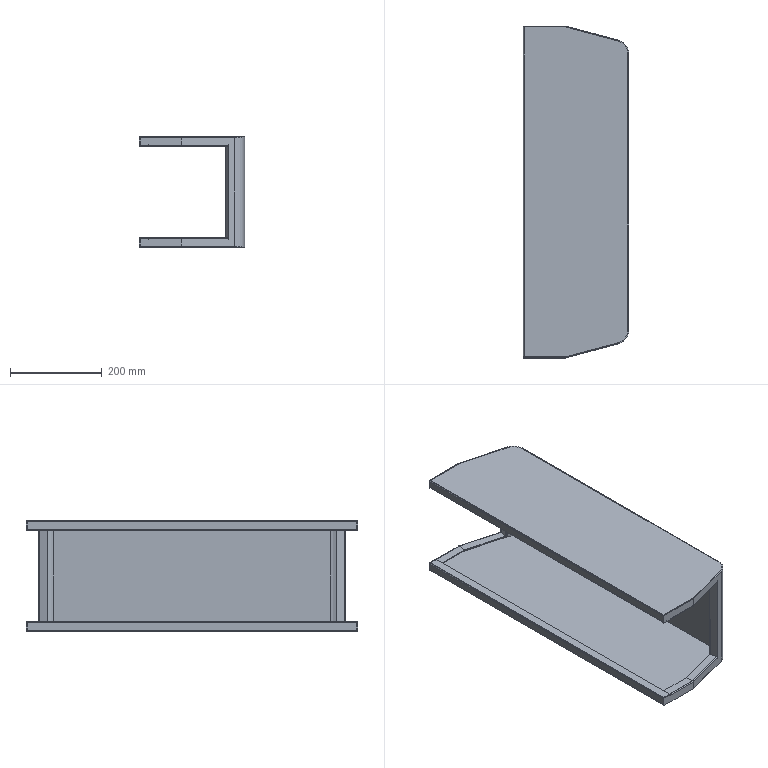Part | SolidWorks | features MirrorCompFeat 2, ReferencePattern 2 | 5 solids | 230 faces | box 229.9 x 723 x 240 mm | volume 1145604 mm3 | plane 182 | cylinder 40 | spline 8 | commonest cylinder face diameters 0.4 x16 4.4 x16 55.8 x6 59.8 x2